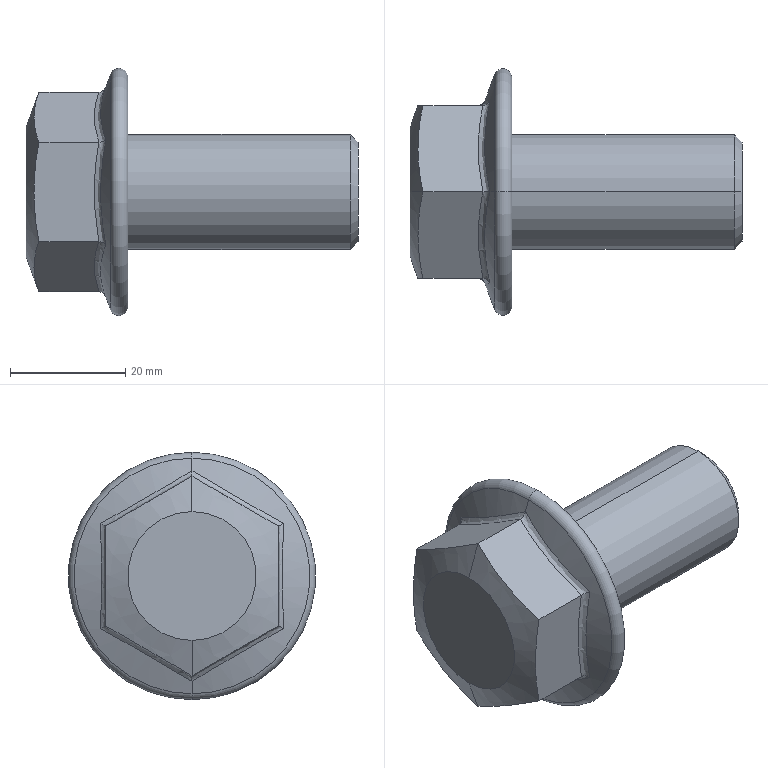Part | SolidWorks | features Fillet 2, RevCut 2, Boss 1, Chamfer 1, Extrusion 1, LPattern 1, Revolution 1 | 1 solid | 25 faces | box 57.7 x 43 x 43 mm | volume 28324 mm3 | plane 9 | cone 6 | spline 6 | torus 2 | cylinder 2 | commonest cylinder face diameters 20 x2
STEP:
#1=CARTESIAN_POINT('',(57.7,0.,-8.647));
#2=VERTEX_POINT('',#1);
#3=CARTESIAN_POINT('',(57.7,0.,8.647));
#4=VERTEX_POINT('',#3);
#5=CARTESIAN_POINT('',(57.7,0.,0.));
#6=DIRECTION('',(1.,0.,0.));
#7=DIRECTION('',(0.,0.,-1.));
#8=AXIS2_PLACEMENT_3D('',#5,#6,#7);
#9=CIRCLE('',#8,8.647);
#10=EDGE_CURVE('',#2,#4,#9,.T.);
#11=ORIENTED_EDGE('',*,*,#10,.F.);
#12=CARTESIAN_POINT('',(56.347,0.,-10.));
#13=VERTEX_POINT('',#12);
#14=CARTESIAN_POINT('',(57.7,0.,-8.647));
#15=DIRECTION('',(-0.7071,0.,-0.7071));
#16=VECTOR('',#15,1000.);
#17=LINE('',#14,#16);
#18=EDGE_CURVE('',#2,#13,#17,.T.);
#19=ORIENTED_EDGE('',*,*,#18,.T.);
#20=CARTESIAN_POINT('',(56.347,0.,10.));
#21=VERTEX_POINT('',#20);
#22=CARTESIAN_POINT('',(56.347,0.,0.));
#23=DIRECTION('',(-1.,0.,0.));
#24=DIRECTION('',(0.,0.,-1.));
#25=AXIS2_PLACEMENT_3D('',#22,#23,#24);
#26=CIRCLE('',#25,10.);
#27=EDGE_CURVE('',#21,#13,#26,.T.);
#28=ORIENTED_EDGE('',*,*,#27,.F.);
#29=CARTESIAN_POINT('',(57.7,0.,8.647));
#30=DIRECTION('',(-0.7071,0.,0.7071));
#31=VECTOR('',#30,1000.);
#32=LINE('',#29,#31);
#33=EDGE_CURVE('',#4,#21,#32,.T.);
#34=ORIENTED_EDGE('',*,*,#33,.F.);
#35=EDGE_LOOP('',(#11,#19,#28,#34));
#36=FACE_OUTER_BOUND('',#35,.T.);
#37=CARTESIAN_POINT('',(57.7,0.,0.));
#38=DIRECTION('',(-1.,0.,0.));
#39=DIRECTION('',(0.,0.,1.));
#40=AXIS2_PLACEMENT_3D('',#37,#38,#39);
#41=CONICAL_SURFACE('',#40,8.647,0.7854);
#42=ADVANCED_FACE('',(#36),#41,.T.);
#43=CARTESIAN_POINT('',(0.,0.,11.2));
#44=VERTEX_POINT('',#43);
#45=CARTESIAN_POINT('',(0.,0.,-11.2));
#46=VERTEX_POINT('',#45);
#47=CARTESIAN_POINT('',(0.,0.,0.));
#48=DIRECTION('',(-1.,0.,0.));
#49=DIRECTION('',(0.,0.,1.));
#50=AXIS2_PLACEMENT_3D('',#47,#48,#49);
#51=CIRCLE('',#50,11.2);
#52=EDGE_CURVE('',#44,#46,#51,.T.);
#53=ORIENTED_EDGE('',*,*,#52,.F.);
#54=CARTESIAN_POINT('',(2.228,0.,17.321));
#55=VERTEX_POINT('',#54);
#56=CARTESIAN_POINT('',(0.,0.,11.2));
#57=DIRECTION('',(0.342,0.,0.9397));
#58=VECTOR('',#57,1000.);
#59=LINE('',#56,#58);
#60=EDGE_CURVE('',#44,#55,#59,.T.);
#61=ORIENTED_EDGE('',*,*,#60,.T.);
#62=CARTESIAN_POINT('',(2.228,15.,8.66));
#63=VERTEX_POINT('',#62);
#64=CARTESIAN_POINT('',(2.228,0.,17.321));
#65=CARTESIAN_POINT('',(1.965,1.25,16.599));
#66=CARTESIAN_POINT('',(1.752,2.5,15.877));
#67=CARTESIAN_POINT('',(1.46,5.,14.434));
#68=CARTESIAN_POINT('',(1.306,7.5,12.99));
#69=CARTESIAN_POINT('',(1.46,10.,11.547));
#70=CARTESIAN_POINT('',(1.752,12.5,10.104));
#71=CARTESIAN_POINT('',(1.965,13.75,9.382));
#72=CARTESIAN_POINT('',(2.228,15.,8.66));
#73=B_SPLINE_CURVE_WITH_KNOTS('',3,(#64,#65,#66,#67,#68,#69,#70,#71,#72),.UNSPECIFIED.,.F.,.F.,(4,2,1,2,4),(0.000000231,0.00433,0.00866,0.01299,0.01732),.UNSPECIFIED.);
#74=EDGE_CURVE('',#55,#63,#73,.T.);
#75=ORIENTED_EDGE('',*,*,#74,.T.);
#76=CARTESIAN_POINT('',(2.228,15.,-8.66));
#77=VERTEX_POINT('',#76);
#78=CARTESIAN_POINT('',(2.228,15.,8.66));
#79=CARTESIAN_POINT('',(1.966,15.,7.223));
#80=CARTESIAN_POINT('',(1.753,15.,5.782));
#81=CARTESIAN_POINT('',(1.461,15.,2.9));
#82=CARTESIAN_POINT('',(1.384,15.,1.458));
#83=CARTESIAN_POINT('',(1.383,15.,-1.431));
#84=CARTESIAN_POINT('',(1.46,15.,-2.877));
#85=CARTESIAN_POINT('',(1.751,15.,-5.773));
#86=CARTESIAN_POINT('',(1.966,15.,-7.224));
#87=CARTESIAN_POINT('',(2.228,15.,-8.66));
#88=B_SPLINE_CURVE_WITH_KNOTS('',3,(#78,#79,#80,#81,#82,#83,#84,#85,#86,#87),.UNSPECIFIED.,.F.,.F.,(4,2,2,2,4),(0.0319,0.03626,0.04061,0.04497,0.04933),.UNSPECIFIED.);
#89=EDGE_CURVE('',#63,#77,#88,.T.);
#90=ORIENTED_EDGE('',*,*,#89,.T.);
#91=CARTESIAN_POINT('',(2.228,0.,-17.321));
#92=VERTEX_POINT('',#91);
#93=CARTESIAN_POINT('',(2.228,15.,-8.66));
#94=CARTESIAN_POINT('',(1.965,13.75,-9.382));
#95=CARTESIAN_POINT('',(1.752,12.5,-10.104));
#96=CARTESIAN_POINT('',(1.46,10.,-11.547));
#97=CARTESIAN_POINT('',(1.306,7.5,-12.99));
#98=CARTESIAN_POINT('',(1.46,5.,-14.434));
#99=CARTESIAN_POINT('',(1.752,2.5,-15.877));
#100=CARTESIAN_POINT('',(1.965,1.25,-16.599));
#101=CARTESIAN_POINT('',(2.228,0.,-17.321));
#102=B_SPLINE_CURVE_WITH_KNOTS('',3,(#93,#94,#95,#96,#97,#98,#99,#100,#101),.UNSPECIFIED.,.F.,.F.,(4,2,1,2,4),(0.000000231,0.00433,0.00866,0.01299,0.01732),.UNSPECIFIED.);
#103=EDGE_CURVE('',#77,#92,#102,.T.);
#104=ORIENTED_EDGE('',*,*,#103,.T.);
#105=CARTESIAN_POINT('',(0.,0.,-11.2));
#106=DIRECTION('',(0.342,0.,-0.9397));
#107=VECTOR('',#106,1000.);
#108=LINE('',#105,#107);
#109=EDGE_CURVE('',#46,#92,#108,.T.);
#110=ORIENTED_EDGE('',*,*,#109,.F.);
#111=EDGE_LOOP('',(#53,#61,#75,#90,#104,#110));
#112=FACE_OUTER_BOUND('',#111,.T.);
#113=CARTESIAN_POINT('',(0.,0.,0.));
#114=DIRECTION('',(1.,0.,0.));
#115=DIRECTION('',(0.,0.,-1.));
#116=AXIS2_PLACEMENT_3D('',#113,#114,#115);
#117=CONICAL_SURFACE('',#116,11.2,1.222);
#118=ADVANCED_FACE('',(#112),#117,.T.);
#119=CARTESIAN_POINT('',(14.7,0.,-20.482));
#120=VERTEX_POINT('',#119);
#121=CARTESIAN_POINT('',(14.7,0.,20.482));
#122=VERTEX_POINT('',#121);
#123=CARTESIAN_POINT('',(14.7,0.,0.));
#124=DIRECTION('',(1.,0.,0.));
#125=DIRECTION('',(0.,0.,-1.));
#126=AXIS2_PLACEMENT_3D('',#123,#124,#125);
#127=CIRCLE('',#126,20.482);
#128=EDGE_CURVE('',#120,#122,#127,.T.);
#129=ORIENTED_EDGE('',*,*,#128,.T.);
#130=CARTESIAN_POINT('',(17.7,0.,19.953));
#131=VERTEX_POINT('',#130);
#132=CARTESIAN_POINT('',(16.153,0.,19.953));
#133=DIRECTION('',(0.,1.,0.));
#134=DIRECTION('',(0.,0.,1.));
#135=AXIS2_PLACEMENT_3D('',#132,#133,#134);
#136=CIRCLE('',#135,1.547);
#137=EDGE_CURVE('',#122,#131,#136,.T.);
#138=ORIENTED_EDGE('',*,*,#137,.T.);
#139=CARTESIAN_POINT('',(17.7,0.,-19.953));
#140=VERTEX_POINT('',#139);
#141=CARTESIAN_POINT('',(17.7,0.,0.));
#142=DIRECTION('',(1.,0.,0.));
#143=DIRECTION('',(0.,0.,-1.));
#144=AXIS2_PLACEMENT_3D('',#141,#142,#143);
#145=CIRCLE('',#144,19.953);
#146=EDGE_CURVE('',#140,#131,#145,.T.);
#147=ORIENTED_EDGE('',*,*,#146,.F.);
#148=CARTESIAN_POINT('',(16.153,0.,-19.953));
#149=DIRECTION('',(0.,-1.,0.));
#150=DIRECTION('',(0.,0.,-1.));
#151=AXIS2_PLACEMENT_3D('',#148,#149,#150);
#152=CIRCLE('',#151,1.547);
#153=EDGE_CURVE('',#120,#140,#152,.T.);
#154=ORIENTED_EDGE('',*,*,#153,.F.);
#155=EDGE_LOOP('',(#129,#138,#147,#154));
#156=FACE_OUTER_BOUND('',#155,.T.);
#157=CARTESIAN_POINT('',(16.153,0.,0.));
#158=DIRECTION('',(1.,0.,0.));
#159=DIRECTION('',(0.,0.,-1.));
#160=AXIS2_PLACEMENT_3D('',#157,#158,#159);
#161=TOROIDAL_SURFACE('',#160,19.953,1.547);
#162=ADVANCED_FACE('',(#156),#161,.T.);
#163=CARTESIAN_POINT('',(13.904,15.845,9.148));
#164=VERTEX_POINT('',#163);
#165=CARTESIAN_POINT('',(13.904,0.,18.296));
#166=VERTEX_POINT('',#165);
#167=CARTESIAN_POINT('',(13.904,15.845,9.148));
#168=CARTESIAN_POINT('',(13.625,14.53,9.89));
#169=CARTESIAN_POINT('',(13.395,13.211,10.636));
#170=CARTESIAN_POINT('',(13.078,10.565,12.14));
#171=CARTESIAN_POINT('',(12.992,9.237,12.899));
#172=CARTESIAN_POINT('',(12.992,6.574,14.437));
#173=CARTESIAN_POINT('',(13.077,5.248,15.209));
#174=CARTESIAN_POINT('',(13.394,2.61,16.756));
#175=CARTESIAN_POINT('',(13.624,1.302,17.527));
#176=CARTESIAN_POINT('',(13.904,0.,18.296));
#177=B_SPLINE_CURVE_WITH_KNOTS('',3,(#167,#168,#169,#170,#171,#172,#173,#174,#175,#176),.UNSPECIFIED.,.F.,.F.,(4,2,2,2,4),(0.,0.004591,0.009181,0.01377,0.01836),.UNSPECIFIED.);
#178=EDGE_CURVE('',#164,#166,#177,.T.);
#179=ORIENTED_EDGE('',*,*,#178,.T.);
#180=CARTESIAN_POINT('',(14.7,0.,20.482));
#181=DIRECTION('',(0.342,0.,0.9397));
#182=VECTOR('',#181,1000.);
#183=LINE('',#180,#182);
#184=EDGE_CURVE('',#166,#122,#183,.T.);
#185=ORIENTED_EDGE('',*,*,#184,.T.);
#186=ORIENTED_EDGE('',*,*,#128,.F.);
#187=CARTESIAN_POINT('',(13.904,0.,-18.296));
#188=VERTEX_POINT('',#187);
#189=CARTESIAN_POINT('',(14.7,0.,-20.482));
#190=DIRECTION('',(0.342,0.,-0.9397));
#191=VECTOR('',#190,1000.);
#192=LINE('',#189,#191);
#193=EDGE_CURVE('',#188,#120,#192,.T.);
#194=ORIENTED_EDGE('',*,*,#193,.F.);
#195=CARTESIAN_POINT('',(13.904,15.845,-9.148));
#196=VERTEX_POINT('',#195);
#197=CARTESIAN_POINT('',(13.904,0.,-18.296));
#198=CARTESIAN_POINT('',(13.625,1.3,-17.528));
#199=CARTESIAN_POINT('',(13.395,2.605,-16.759));
#200=CARTESIAN_POINT('',(13.078,5.231,-15.219));
#201=CARTESIAN_POINT('',(12.992,6.552,-14.449));
#202=CARTESIAN_POINT('',(12.992,9.216,-12.911));
#203=CARTESIAN_POINT('',(13.077,10.547,-12.15));
#204=CARTESIAN_POINT('',(13.394,13.206,-10.638));
#205=CARTESIAN_POINT('',(13.624,14.528,-9.891));
#206=CARTESIAN_POINT('',(13.904,15.845,-9.148));
#207=B_SPLINE_CURVE_WITH_KNOTS('',3,(#197,#198,#199,#200,#201,#202,#203,#204,#205,#206),.UNSPECIFIED.,.F.,.F.,(4,2,2,2,4),(0.,0.004591,0.009181,0.01377,0.01836),.UNSPECIFIED.);
#208=EDGE_CURVE('',#188,#196,#207,.T.);
#209=ORIENTED_EDGE('',*,*,#208,.T.);
#210=CARTESIAN_POINT('',(13.904,15.845,-9.148));
#211=CARTESIAN_POINT('',(13.625,15.83,-7.638));
#212=CARTESIAN_POINT('',(13.395,15.816,-6.123));
#213=CARTESIAN_POINT('',(13.078,15.796,-3.079));
#214=CARTESIAN_POINT('',(12.992,15.79,-1.55));
#215=CARTESIAN_POINT('',(12.992,15.79,1.525));
#216=CARTESIAN_POINT('',(13.077,15.796,3.059));
#217=CARTESIAN_POINT('',(13.394,15.816,6.118));
#218=CARTESIAN_POINT('',(13.624,15.83,7.636));
#219=CARTESIAN_POINT('',(13.904,15.845,9.148));
#220=B_SPLINE_CURVE_WITH_KNOTS('',3,(#210,#211,#212,#213,#214,#215,#216,#217,#218,#219),.UNSPECIFIED.,.F.,.F.,(4,2,2,2,4),(0.,0.00459,0.009181,0.01377,0.01836),.UNSPECIFIED.);
#221=EDGE_CURVE('',#196,#164,#220,.T.);
#222=ORIENTED_EDGE('',*,*,#221,.T.);
#223=EDGE_LOOP('',(#179,#185,#186,#194,#209,#222));
#224=FACE_OUTER_BOUND('',#223,.T.);
#225=CARTESIAN_POINT('',(14.7,0.,0.));
#226=DIRECTION('',(1.,0.,0.));
#227=DIRECTION('',(0.,0.,-1.));
#228=AXIS2_PLACEMENT_3D('',#225,#226,#227);
#229=CONICAL_SURFACE('',#228,20.482,1.222);
#230=ADVANCED_FACE('',(#224),#229,.T.);
#231=ORIENTED_EDGE('',*,*,#27,.T.);
#232=CARTESIAN_POINT('',(17.7,0.,-10.));
#233=VERTEX_POINT('',#232);
#234=CARTESIAN_POINT('',(57.7,0.,-10.));
#235=DIRECTION('',(-1.,0.,0.));
#236=VECTOR('',#235,1000.);
#237=LINE('',#234,#236);
#238=EDGE_CURVE('',#13,#233,#237,.T.);
#239=ORIENTED_EDGE('',*,*,#238,.T.);
#240=CARTESIAN_POINT('',(17.7,0.,10.));
#241=VERTEX_POINT('',#240);
#242=CARTESIAN_POINT('',(17.7,0.,0.));
#243=DIRECTION('',(1.,0.,0.));
#244=DIRECTION('',(0.,0.,-1.));
#245=AXIS2_PLACEMENT_3D('',#242,#243,#244);
#246=CIRCLE('',#245,10.);
#247=EDGE_CURVE('',#233,#241,#246,.T.);
#248=ORIENTED_EDGE('',*,*,#247,.T.);
#249=CARTESIAN_POINT('',(57.7,0.,10.));
#250=DIRECTION('',(-1.,0.,0.));
#251=VECTOR('',#250,1000.);
#252=LINE('',#249,#251);
#253=EDGE_CURVE('',#21,#241,#252,.T.);
#254=ORIENTED_EDGE('',*,*,#253,.F.);
#255=EDGE_LOOP('',(#231,#239,#248,#254));
#256=FACE_OUTER_BOUND('',#255,.T.);
#257=CARTESIAN_POINT('',(57.7,0.,0.));
#258=DIRECTION('',(-1.,0.,0.));
#259=DIRECTION('',(0.,0.,1.));
#260=AXIS2_PLACEMENT_3D('',#257,#258,#259);
#261=CYLINDRICAL_SURFACE('',#260,10.);
#262=ADVANCED_FACE('',(#256),#261,.T.);
#263=CARTESIAN_POINT('',(17.7,0.,0.));
#264=DIRECTION('',(1.,0.,0.));
#265=DIRECTION('',(0.,0.,-1.));
#266=AXIS2_PLACEMENT_3D('',#263,#264,#265);
#267=CIRCLE('',#266,10.);
#268=EDGE_CURVE('',#241,#233,#267,.T.);
#269=ORIENTED_EDGE('',*,*,#268,.F.);
#270=ORIENTED_EDGE('',*,*,#247,.F.);
#271=EDGE_LOOP('',(#269,#270));
#272=FACE_BOUND('',#271,.T.);
#273=ORIENTED_EDGE('',*,*,#146,.T.);
#274=CARTESIAN_POINT('',(17.7,0.,0.));
#275=DIRECTION('',(1.,0.,0.));
#276=DIRECTION('',(0.,0.,-1.));
#277=AXIS2_PLACEMENT_3D('',#274,#275,#276);
#278=CIRCLE('',#277,19.953);
#279=EDGE_CURVE('',#131,#140,#278,.T.);
#280=ORIENTED_EDGE('',*,*,#279,.T.);
#281=EDGE_LOOP('',(#273,#280));
#282=FACE_OUTER_BOUND('',#281,.T.);
#283=CARTESIAN_POINT('',(17.7,0.,-17.321));
#284=DIRECTION('',(1.,0.,0.));
#285=DIRECTION('',(0.,0.,-1.));
#286=AXIS2_PLACEMENT_3D('',#283,#284,#285);
#287=PLANE('',#286);
#288=ADVANCED_FACE('',(#272,#282),#287,.T.);
#289=ORIENTED_EDGE('',*,*,#238,.F.);
#290=CARTESIAN_POINT('',(56.347,0.,0.));
#291=DIRECTION('',(-1.,0.,0.));
#292=DIRECTION('',(0.,0.,-1.));
#293=AXIS2_PLACEMENT_3D('',#290,#291,#292);
#294=CIRCLE('',#293,10.);
#295=EDGE_CURVE('',#13,#21,#294,.T.);
#296=ORIENTED_EDGE('',*,*,#295,.T.);
#297=ORIENTED_EDGE('',*,*,#253,.T.);
#298=ORIENTED_EDGE('',*,*,#268,.T.);
#299=EDGE_LOOP('',(#289,#296,#297,#298));
#300=FACE_OUTER_BOUND('',#299,.T.);
#301=CARTESIAN_POINT('',(57.7,0.,0.));
#302=DIRECTION('',(-1.,0.,0.));
#303=DIRECTION('',(0.,0.,1.));
#304=AXIS2_PLACEMENT_3D('',#301,#302,#303);
#305=CYLINDRICAL_SURFACE('',#304,10.);
#306=ADVANCED_FACE('',(#300),#305,.T.);
#307=CARTESIAN_POINT('',(57.7,0.,0.));
#308=DIRECTION('',(1.,0.,0.));
#309=DIRECTION('',(0.,0.,-1.));
#310=AXIS2_PLACEMENT_3D('',#307,#308,#309);
#311=CIRCLE('',#310,8.647);
#312=EDGE_CURVE('',#4,#2,#311,.T.);
#313=ORIENTED_EDGE('',*,*,#312,.T.);
#314=ORIENTED_EDGE('',*,*,#10,.T.);
#315=EDGE_LOOP('',(#313,#314));
#316=FACE_OUTER_BOUND('',#315,.T.);
#317=CARTESIAN_POINT('',(57.7,0.,0.));
#318=DIRECTION('',(1.,0.,0.));
#319=DIRECTION('',(0.,0.,-1.));
#320=AXIS2_PLACEMENT_3D('',#317,#318,#319);
#321=PLANE('',#320);
#322=ADVANCED_FACE('',(#316),#321,.T.);
#323=ORIENTED_EDGE('',*,*,#184,.F.);
#324=CARTESIAN_POINT('',(13.904,-15.845,9.148));
#325=VERTEX_POINT('',#324);
#326=CARTESIAN_POINT('',(13.904,0.,18.296));
#327=CARTESIAN_POINT('',(13.625,-1.3,17.528));
#328=CARTESIAN_POINT('',(13.395,-2.605,16.759));
#329=CARTESIAN_POINT('',(13.078,-5.231,15.219));
#330=CARTESIAN_POINT('',(12.992,-6.552,14.449));
#331=CARTESIAN_POINT('',(12.992,-9.216,12.911));
#332=CARTESIAN_POINT('',(13.077,-10.547,12.15));
#333=CARTESIAN_POINT('',(13.394,-13.206,10.638));
#334=CARTESIAN_POINT('',(13.624,-14.528,9.891));
#335=CARTESIAN_POINT('',(13.904,-15.845,9.148));
#336=B_SPLINE_CURVE_WITH_KNOTS('',3,(#326,#327,#328,#329,#330,#331,#332,#333,#334,#335),.UNSPECIFIED.,.F.,.F.,(4,2,2,2,4),(0.,0.004591,0.009181,0.01377,0.01836),.UNSPECIFIED.);
#337=EDGE_CURVE('',#166,#325,#336,.T.);
#338=ORIENTED_EDGE('',*,*,#337,.T.);
#339=CARTESIAN_POINT('',(13.904,-15.845,-9.148));
#340=VERTEX_POINT('',#339);
#341=CARTESIAN_POINT('',(13.904,-15.845,9.148));
#342=CARTESIAN_POINT('',(13.625,-15.83,7.638));
#343=CARTESIAN_POINT('',(13.395,-15.816,6.123));
#344=CARTESIAN_POINT('',(13.078,-15.796,3.079));
#345=CARTESIAN_POINT('',(12.992,-15.79,1.55));
#346=CARTESIAN_POINT('',(12.992,-15.79,-1.525));
#347=CARTESIAN_POINT('',(13.077,-15.796,-3.06));
#348=CARTESIAN_POINT('',(13.394,-15.816,-6.118));
#349=CARTESIAN_POINT('',(13.624,-15.83,-7.636));
#350=CARTESIAN_POINT('',(13.904,-15.845,-9.148));
#351=B_SPLINE_CURVE_WITH_KNOTS('',3,(#341,#342,#343,#344,#345,#346,#347,#348,#349,#350),.UNSPECIFIED.,.F.,.F.,(4,2,2,2,4),(0.,0.004591,0.009181,0.01377,0.01836),.UNSPECIFIED.);
#352=EDGE_CURVE('',#325,#340,#351,.T.);
#353=ORIENTED_EDGE('',*,*,#352,.T.);
#354=CARTESIAN_POINT('',(13.904,-15.845,-9.148));
#355=CARTESIAN_POINT('',(13.625,-14.53,-9.89));
#356=CARTESIAN_POINT('',(13.395,-13.211,-10.636));
#357=CARTESIAN_POINT('',(13.078,-10.565,-12.14));
#358=CARTESIAN_POINT('',(12.992,-9.237,-12.899));
#359=CARTESIAN_POINT('',(12.992,-6.574,-14.437));
#360=CARTESIAN_POINT('',(13.077,-5.248,-15.209));
#361=CARTESIAN_POINT('',(13.394,-2.61,-16.756));
#362=CARTESIAN_POINT('',(13.624,-1.302,-17.527));
#363=CARTESIAN_POINT('',(13.904,0.,-18.296));
#364=B_SPLINE_CURVE_WITH_KNOTS('',3,(#354,#355,#356,#357,#358,#359,#360,#361,#362,#363),.UNSPECIFIED.,.F.,.F.,(4,2,2,2,4),(0.,0.004591,0.009181,0.01377,0.01836),.UNSPECIFIED.);
#365=EDGE_CURVE('',#340,#188,#364,.T.);
#366=ORIENTED_EDGE('',*,*,#365,.T.);
#367=ORIENTED_EDGE('',*,*,#193,.T.);
#368=CARTESIAN_POINT('',(14.7,0.,0.));
#369=DIRECTION('',(1.,0.,0.));
#370=DIRECTION('',(0.,0.,-1.));
#371=AXIS2_PLACEMENT_3D('',#368,#369,#370);
#372=CIRCLE('',#371,20.482);
#373=EDGE_CURVE('',#122,#120,#372,.T.);
#374=ORIENTED_EDGE('',*,*,#373,.F.);
#375=EDGE_LOOP('',(#323,#338,#353,#366,#367,#374));
#376=FACE_OUTER_BOUND('',#375,.T.);
#377=CARTESIAN_POINT('',(14.7,0.,0.));
#378=DIRECTION('',(1.,0.,0.));
#379=DIRECTION('',(0.,0.,-1.));
#380=AXIS2_PLACEMENT_3D('',#377,#378,#379);
#381=CONICAL_SURFACE('',#380,20.482,1.222);
#382=ADVANCED_FACE('',(#376),#381,.T.);
#383=ORIENTED_EDGE('',*,*,#137,.F.);
#384=ORIENTED_EDGE('',*,*,#373,.T.);
#385=ORIENTED_EDGE('',*,*,#153,.T.);
#386=ORIENTED_EDGE('',*,*,#279,.F.);
#387=EDGE_LOOP('',(#383,#384,#385,#386));
#388=FACE_OUTER_BOUND('',#387,.T.);
#389=CARTESIAN_POINT('',(16.153,0.,0.));
#390=DIRECTION('',(1.,0.,0.));
#391=DIRECTION('',(0.,0.,-1.));
#392=AXIS2_PLACEMENT_3D('',#389,#390,#391);
#393=TOROIDAL_SURFACE('',#392,19.953,1.547);
#394=ADVANCED_FACE('',(#388),#393,.T.);
#395=CARTESIAN_POINT('',(0.,0.,0.));
#396=DIRECTION('',(-1.,0.,0.));
#397=DIRECTION('',(0.,0.,1.));
#398=AXIS2_PLACEMENT_3D('',#395,#396,#397);
#399=CIRCLE('',#398,11.2);
#400=EDGE_CURVE('',#46,#44,#399,.T.);
#401=ORIENTED_EDGE('',*,*,#400,.T.);
#402=ORIENTED_EDGE('',*,*,#52,.T.);
#403=EDGE_LOOP('',(#401,#402));
#404=FACE_OUTER_BOUND('',#403,.T.);
#405=CARTESIAN_POINT('',(0.,0.,-17.321));
#406=DIRECTION('',(1.,0.,0.));
#407=DIRECTION('',(0.,0.,-1.));
#408=AXIS2_PLACEMENT_3D('',#405,#406,#407);
#409=PLANE('',#408);
#410=ADVANCED_FACE('',(#404),#409,.F.);
#411=ORIENTED_EDGE('',*,*,#60,.F.);
#412=ORIENTED_EDGE('',*,*,#400,.F.);
#413=ORIENTED_EDGE('',*,*,#109,.T.);
#414=CARTESIAN_POINT('',(2.228,-15.,-8.66));
#415=VERTEX_POINT('',#414);
#416=CARTESIAN_POINT('',(2.228,0.,-17.321));
#417=CARTESIAN_POINT('',(1.965,-1.25,-16.599));
#418=CARTESIAN_POINT('',(1.752,-2.5,-15.877));
#419=CARTESIAN_POINT('',(1.46,-5.,-14.434));
#420=CARTESIAN_POINT('',(1.306,-7.5,-12.99));
#421=CARTESIAN_POINT('',(1.46,-10.,-11.547));
#422=CARTESIAN_POINT('',(1.752,-12.5,-10.104));
#423=CARTESIAN_POINT('',(1.965,-13.75,-9.382));
#424=CARTESIAN_POINT('',(2.228,-15.,-8.66));
#425=B_SPLINE_CURVE_WITH_KNOTS('',3,(#416,#417,#418,#419,#420,#421,#422,#423,#424),.UNSPECIFIED.,.F.,.F.,(4,2,1,2,4),(0.000000231,0.00433,0.00866,0.01299,0.01732),.UNSPECIFIED.);
#426=EDGE_CURVE('',#92,#415,#425,.T.);
#427=ORIENTED_EDGE('',*,*,#426,.T.);
#428=CARTESIAN_POINT('',(2.228,-15.,8.66));
#429=VERTEX_POINT('',#428);
#430=CARTESIAN_POINT('',(2.228,-15.,-8.66));
#431=CARTESIAN_POINT('',(1.966,-15.,-7.224));
#432=CARTESIAN_POINT('',(1.751,-15.,-5.773));
#433=CARTESIAN_POINT('',(1.46,-15.,-2.877));
#434=CARTESIAN_POINT('',(1.383,-15.,-1.431));
#435=CARTESIAN_POINT('',(1.384,-15.,1.458));
#436=CARTESIAN_POINT('',(1.461,-15.,2.9));
#437=CARTESIAN_POINT('',(1.753,-15.,5.782));
#438=CARTESIAN_POINT('',(1.966,-15.,7.223));
#439=CARTESIAN_POINT('',(2.228,-15.,8.66));
#440=B_SPLINE_CURVE_WITH_KNOTS('',3,(#430,#431,#432,#433,#434,#435,#436,#437,#438,#439),.UNSPECIFIED.,.F.,.F.,(4,2,2,2,4),(0.01459,0.01897,0.02334,0.02771,0.03208),.UNSPECIFIED.);
#441=EDGE_CURVE('',#415,#429,#440,.T.);
#442=ORIENTED_EDGE('',*,*,#441,.T.);
#443=CARTESIAN_POINT('',(2.228,-15.,8.66));
#444=CARTESIAN_POINT('',(1.965,-13.75,9.382));
#445=CARTESIAN_POINT('',(1.752,-12.5,10.104));
#446=CARTESIAN_POINT('',(1.46,-10.,11.547));
#447=CARTESIAN_POINT('',(1.306,-7.5,12.99));
#448=CARTESIAN_POINT('',(1.46,-5.,14.434));
#449=CARTESIAN_POINT('',(1.752,-2.5,15.877));
#450=CARTESIAN_POINT('',(1.965,-1.25,16.599));
#451=CARTESIAN_POINT('',(2.228,0.,17.321));
#452=B_SPLINE_CURVE_WITH_KNOTS('',3,(#443,#444,#445,#446,#447,#448,#449,#450,#451),.UNSPECIFIED.,.F.,.F.,(4,2,1,2,4),(0.000000231,0.00433,0.00866,0.01299,0.01732),.UNSPECIFIED.);
#453=EDGE_CURVE('',#429,#55,#452,.T.);
#454=ORIENTED_EDGE('',*,*,#453,.T.);
#455=EDGE_LOOP('',(#411,#412,#413,#427,#442,#454));
#456=FACE_OUTER_BOUND('',#455,.T.);
#457=CARTESIAN_POINT('',(0.,0.,0.));
#458=DIRECTION('',(1.,0.,0.));
#459=DIRECTION('',(0.,0.,-1.));
#460=AXIS2_PLACEMENT_3D('',#457,#458,#459);
#461=CONICAL_SURFACE('',#460,11.2,1.222);
#462=ADVANCED_FACE('',(#456),#461,.T.);
#463=CARTESIAN_POINT('',(12.654,-15.,-8.66));
#464=VERTEX_POINT('',#463);
#465=CARTESIAN_POINT('',(17.7,-15.,-8.66));
#466=DIRECTION('',(-1.,0.,0.));
#467=VECTOR('',#466,1000.);
#468=LINE('',#465,#467);
#469=EDGE_CURVE('',#464,#415,#468,.T.);
#470=ORIENTED_EDGE('',*,*,#469,.F.);
#471=CARTESIAN_POINT('',(12.654,-15.,8.66));
#472=VERTEX_POINT('',#471);
#473=CARTESIAN_POINT('',(12.654,-15.,-8.66));
#474=CARTESIAN_POINT('',(12.408,-15.,-7.227));
#475=CARTESIAN_POINT('',(12.209,-15.,-5.79));
#476=CARTESIAN_POINT('',(11.937,-15.,-2.904));
#477=CARTESIAN_POINT('',(11.864,-15.,-1.455));
#478=CARTESIAN_POINT('',(11.864,-15.,1.455));
#479=CARTESIAN_POINT('',(11.937,-15.,2.904));
#480=CARTESIAN_POINT('',(12.209,-15.,5.79));
#481=CARTESIAN_POINT('',(12.408,-15.,7.227));
#482=CARTESIAN_POINT('',(12.654,-15.,8.66));
#483=B_SPLINE_CURVE_WITH_KNOTS('',3,(#473,#474,#475,#476,#477,#478,#479,#480,#481,#482),.UNSPECIFIED.,.F.,.F.,(4,2,2,2,4),(0.,0.004348,0.008696,0.01304,0.01739),.UNSPECIFIED.);
#484=EDGE_CURVE('',#464,#472,#483,.T.);
#485=ORIENTED_EDGE('',*,*,#484,.T.);
#486=CARTESIAN_POINT('',(17.7,-15.,8.66));
#487=DIRECTION('',(-1.,0.,0.));
#488=VECTOR('',#487,1000.);
#489=LINE('',#486,#488);
#490=EDGE_CURVE('',#472,#429,#489,.T.);
#491=ORIENTED_EDGE('',*,*,#490,.T.);
#492=ORIENTED_EDGE('',*,*,#441,.F.);
#493=EDGE_LOOP('',(#470,#485,#491,#492));
#494=FACE_OUTER_BOUND('',#493,.T.);
#495=CARTESIAN_POINT('',(17.7,-15.,8.66));
#496=DIRECTION('',(0.,1.,0.));
#497=DIRECTION('',(0.,0.,1.));
#498=AXIS2_PLACEMENT_3D('',#495,#496,#497);
#499=PLANE('',#498);
#500=ADVANCED_FACE('',(#494),#499,.F.);
#501=ORIENTED_EDGE('',*,*,#490,.F.);
#502=CARTESIAN_POINT('',(12.654,0.,17.321));
#503=VERTEX_POINT('',#502);
#504=CARTESIAN_POINT('',(12.654,-15.,8.66));
#505=CARTESIAN_POINT('',(12.408,-13.759,9.377));
#506=CARTESIAN_POINT('',(12.209,-12.514,10.095));
#507=CARTESIAN_POINT('',(11.937,-10.015,11.538));
#508=CARTESIAN_POINT('',(11.864,-8.76,12.263));
#509=CARTESIAN_POINT('',(11.864,-6.24,13.718));
#510=CARTESIAN_POINT('',(11.937,-4.985,14.442));
#511=CARTESIAN_POINT('',(12.209,-2.486,15.885));
#512=CARTESIAN_POINT('',(12.408,-1.241,16.604));
#513=CARTESIAN_POINT('',(12.654,0.,17.321));
#514=B_SPLINE_CURVE_WITH_KNOTS('',3,(#504,#505,#506,#507,#508,#509,#510,#511,#512,#513),.UNSPECIFIED.,.F.,.F.,(4,2,2,2,4),(0.,0.004348,0.008696,0.01304,0.01739),.UNSPECIFIED.);
#515=EDGE_CURVE('',#472,#503,#514,.T.);
#516=ORIENTED_EDGE('',*,*,#515,.T.);
#517=CARTESIAN_POINT('',(17.7,0.,17.321));
#518=DIRECTION('',(-1.,0.,0.));
#519=VECTOR('',#518,1000.);
#520=LINE('',#517,#519);
#521=EDGE_CURVE('',#503,#55,#520,.T.);
#522=ORIENTED_EDGE('',*,*,#521,.T.);
#523=ORIENTED_EDGE('',*,*,#453,.F.);
#524=EDGE_LOOP('',(#501,#516,#522,#523));
#525=FACE_OUTER_BOUND('',#524,.T.);
#526=CARTESIAN_POINT('',(17.7,0.,17.321));
#527=DIRECTION('',(0.,0.5,-0.866));
#528=DIRECTION('',(0.,0.866,0.5));
#529=AXIS2_PLACEMENT_3D('',#526,#527,#528);
#530=PLANE('',#529);
#531=ADVANCED_FACE('',(#525),#530,.F.);
#532=ORIENTED_EDGE('',*,*,#521,.F.);
#533=CARTESIAN_POINT('',(12.654,15.,8.66));
#534=VERTEX_POINT('',#533);
#535=CARTESIAN_POINT('',(12.654,0.,17.321));
#536=CARTESIAN_POINT('',(12.408,1.241,16.604));
#537=CARTESIAN_POINT('',(12.209,2.486,15.885));
#538=CARTESIAN_POINT('',(11.937,4.985,14.442));
#539=CARTESIAN_POINT('',(11.864,6.24,13.718));
#540=CARTESIAN_POINT('',(11.864,8.76,12.263));
#541=CARTESIAN_POINT('',(11.937,10.015,11.538));
#542=CARTESIAN_POINT('',(12.209,12.514,10.095));
#543=CARTESIAN_POINT('',(12.408,13.759,9.377));
#544=CARTESIAN_POINT('',(12.654,15.,8.66));
#545=B_SPLINE_CURVE_WITH_KNOTS('',3,(#535,#536,#537,#538,#539,#540,#541,#542,#543,#544),.UNSPECIFIED.,.F.,.F.,(4,2,2,2,4),(0.,0.004348,0.008696,0.01304,0.01739),.UNSPECIFIED.);
#546=EDGE_CURVE('',#503,#534,#545,.T.);
#547=ORIENTED_EDGE('',*,*,#546,.T.);
#548=CARTESIAN_POINT('',(17.7,15.,8.66));
#549=DIRECTION('',(-1.,0.,0.));
#550=VECTOR('',#549,1000.);
#551=LINE('',#548,#550);
#552=EDGE_CURVE('',#534,#63,#551,.T.);
#553=ORIENTED_EDGE('',*,*,#552,.T.);
#554=ORIENTED_EDGE('',*,*,#74,.F.);
#555=EDGE_LOOP('',(#532,#547,#553,#554));
#556=FACE_OUTER_BOUND('',#555,.T.);
#557=CARTESIAN_POINT('',(17.7,15.,8.66));
#558=DIRECTION('',(0.,-0.5,-0.866));
#559=DIRECTION('',(0.,0.866,-0.5));
#560=AXIS2_PLACEMENT_3D('',#557,#558,#559);
#561=PLANE('',#560);
#562=ADVANCED_FACE('',(#556),#561,.F.);
#563=ORIENTED_EDGE('',*,*,#552,.F.);
#564=CARTESIAN_POINT('',(12.654,15.,-8.66));
#565=VERTEX_POINT('',#564);
#566=CARTESIAN_POINT('',(12.654,15.,8.66));
#567=CARTESIAN_POINT('',(12.408,15.,7.227));
#568=CARTESIAN_POINT('',(12.209,15.,5.79));
#569=CARTESIAN_POINT('',(11.937,15.,2.904));
#570=CARTESIAN_POINT('',(11.864,15.,1.455));
#571=CARTESIAN_POINT('',(11.864,15.,-1.455));
#572=CARTESIAN_POINT('',(11.937,15.,-2.904));
#573=CARTESIAN_POINT('',(12.209,15.,-5.79));
#574=CARTESIAN_POINT('',(12.408,15.,-7.227));
#575=CARTESIAN_POINT('',(12.654,15.,-8.66));
#576=B_SPLINE_CURVE_WITH_KNOTS('',3,(#566,#567,#568,#569,#570,#571,#572,#573,#574,#575),.UNSPECIFIED.,.F.,.F.,(4,2,2,2,4),(0.,0.004348,0.008696,0.01304,0.01739),.UNSPECIFIED.);
#577=EDGE_CURVE('',#534,#565,#576,.T.);
#578=ORIENTED_EDGE('',*,*,#577,.T.);
#579=CARTESIAN_POINT('',(17.7,15.,-8.66));
#580=DIRECTION('',(-1.,0.,0.));
#581=VECTOR('',#580,1000.);
#582=LINE('',#579,#581);
#583=EDGE_CURVE('',#565,#77,#582,.T.);
#584=ORIENTED_EDGE('',*,*,#583,.T.);
#585=ORIENTED_EDGE('',*,*,#89,.F.);
#586=EDGE_LOOP('',(#563,#578,#584,#585));
#587=FACE_OUTER_BOUND('',#586,.T.);
#588=CARTESIAN_POINT('',(17.7,15.,-8.66));
#589=DIRECTION('',(0.,-1.,0.));
#590=DIRECTION('',(0.,0.,-1.));
#591=AXIS2_PLACEMENT_3D('',#588,#589,#590);
#592=PLANE('',#591);
#593=ADVANCED_FACE('',(#587),#592,.F.);
#594=ORIENTED_EDGE('',*,*,#583,.F.);
#595=CARTESIAN_POINT('',(12.654,0.,-17.321));
#596=VERTEX_POINT('',#595);
#597=CARTESIAN_POINT('',(12.654,15.,-8.66));
#598=CARTESIAN_POINT('',(12.408,13.759,-9.377));
#599=CARTESIAN_POINT('',(12.209,12.514,-10.095));
#600=CARTESIAN_POINT('',(11.937,10.015,-11.538));
#601=CARTESIAN_POINT('',(11.864,8.76,-12.263));
#602=CARTESIAN_POINT('',(11.864,6.24,-13.718));
#603=CARTESIAN_POINT('',(11.937,4.985,-14.442));
#604=CARTESIAN_POINT('',(12.209,2.486,-15.885));
#605=CARTESIAN_POINT('',(12.408,1.241,-16.604));
#606=CARTESIAN_POINT('',(12.654,0.,-17.321));
#607=B_SPLINE_CURVE_WITH_KNOTS('',3,(#597,#598,#599,#600,#601,#602,#603,#604,#605,#606),.UNSPECIFIED.,.F.,.F.,(4,2,2,2,4),(0.,0.004348,0.008696,0.01304,0.01739),.UNSPECIFIED.);
#608=EDGE_CURVE('',#565,#596,#607,.T.);
#609=ORIENTED_EDGE('',*,*,#608,.T.);
#610=CARTESIAN_POINT('',(17.7,0.,-17.321));
#611=DIRECTION('',(-1.,0.,0.));
#612=VECTOR('',#611,1000.);
#613=LINE('',#610,#612);
#614=EDGE_CURVE('',#596,#92,#613,.T.);
#615=ORIENTED_EDGE('',*,*,#614,.T.);
#616=ORIENTED_EDGE('',*,*,#103,.F.);
#617=EDGE_LOOP('',(#594,#609,#615,#616));
#618=FACE_OUTER_BOUND('',#617,.T.);
#619=CARTESIAN_POINT('',(17.7,0.,-17.321));
#620=DIRECTION('',(0.,-0.5,0.866));
#621=DIRECTION('',(0.,-0.866,-0.5));
#622=AXIS2_PLACEMENT_3D('',#619,#620,#621);
#623=PLANE('',#622);
#624=ADVANCED_FACE('',(#618),#623,.F.);
#625=ORIENTED_EDGE('',*,*,#614,.F.);
#626=CARTESIAN_POINT('',(12.654,0.,-17.321));
#627=CARTESIAN_POINT('',(12.408,-1.241,-16.604));
#628=CARTESIAN_POINT('',(12.209,-2.486,-15.885));
#629=CARTESIAN_POINT('',(11.937,-4.985,-14.442));
#630=CARTESIAN_POINT('',(11.864,-6.24,-13.718));
#631=CARTESIAN_POINT('',(11.864,-8.76,-12.263));
#632=CARTESIAN_POINT('',(11.937,-10.015,-11.538));
#633=CARTESIAN_POINT('',(12.209,-12.514,-10.095));
#634=CARTESIAN_POINT('',(12.408,-13.759,-9.377));
#635=CARTESIAN_POINT('',(12.654,-15.,-8.66));
#636=B_SPLINE_CURVE_WITH_KNOTS('',3,(#626,#627,#628,#629,#630,#631,#632,#633,#634,#635),.UNSPECIFIED.,.F.,.F.,(4,2,2,2,4),(0.,0.004348,0.008696,0.01304,0.01739),.UNSPECIFIED.);
#637=EDGE_CURVE('',#596,#464,#636,.T.);
#638=ORIENTED_EDGE('',*,*,#637,.T.);
#639=ORIENTED_EDGE('',*,*,#469,.T.);
#640=ORIENTED_EDGE('',*,*,#426,.F.);
#641=EDGE_LOOP('',(#625,#638,#639,#640));
#642=FACE_OUTER_BOUND('',#641,.T.);
#643=CARTESIAN_POINT('',(17.7,-15.,-8.66));
#644=DIRECTION('',(0.,0.5,0.866));
#645=DIRECTION('',(0.,-0.866,0.5));
#646=AXIS2_PLACEMENT_3D('',#643,#644,#645);
#647=PLANE('',#646);
#648=ADVANCED_FACE('',(#642),#647,.F.);
#649=CARTESIAN_POINT('',(13.904,0.,-18.296));
#650=CARTESIAN_POINT('',(13.808,0.,-18.032));
#651=CARTESIAN_POINT('',(13.645,0.,-17.791));
#652=CARTESIAN_POINT('',(13.209,0.,-17.434));
#653=CARTESIAN_POINT('',(12.938,0.,-17.321));
#654=CARTESIAN_POINT('',(12.654,0.,-17.321));
#655=B_SPLINE_CURVE_WITH_KNOTS('',3,(#649,#650,#651,#652,#653,#654),.UNSPECIFIED.,.F.,.F.,(4,2,4),(-0.000007277,0.0008336,0.001674),.UNSPECIFIED.);
#656=EDGE_CURVE('',#188,#596,#655,.T.);
#657=ORIENTED_EDGE('',*,*,#656,.F.);
#658=ORIENTED_EDGE('',*,*,#365,.F.);
#659=CARTESIAN_POINT('',(12.654,-15.,-8.66));
#660=CARTESIAN_POINT('',(12.938,-15.,-8.66));
#661=CARTESIAN_POINT('',(13.209,-15.098,-8.717));
#662=CARTESIAN_POINT('',(13.536,-15.33,-8.851));
#663=CARTESIAN_POINT('',(13.631,-15.421,-8.903));
#664=CARTESIAN_POINT('',(13.792,-15.622,-9.019));
#665=CARTESIAN_POINT('',(13.856,-15.731,-9.082));
#666=CARTESIAN_POINT('',(13.904,-15.845,-9.148));
#667=B_SPLINE_CURVE_WITH_KNOTS('',3,(#659,#660,#661,#662,#663,#664,#665,#666),.UNSPECIFIED.,.F.,.F.,(4,2,2,4),(0.,0.000838,0.001257,0.001676),.UNSPECIFIED.);
#668=EDGE_CURVE('',#464,#340,#667,.T.);
#669=ORIENTED_EDGE('',*,*,#668,.F.);
#670=ORIENTED_EDGE('',*,*,#637,.F.);
#671=EDGE_LOOP('',(#657,#658,#669,#670));
#672=FACE_OUTER_BOUND('',#671,.T.);
#673=CARTESIAN_POINT('',(12.796,0.6942,-17.721));
#674=CARTESIAN_POINT('',(13.667,0.5558,-17.641));
#675=CARTESIAN_POINT('',(13.924,0.09214,-18.35));
#676=CARTESIAN_POINT('',(12.516,-0.6296,-16.957));
#677=CARTESIAN_POINT('',(13.379,-0.744,-16.891));
#678=CARTESIAN_POINT('',(13.643,-1.203,-17.586));
#679=CARTESIAN_POINT('',(12.283,-1.966,-16.186));
#680=CARTESIAN_POINT('',(13.138,-2.061,-16.131));
#681=CARTESIAN_POINT('',(13.411,-2.506,-16.817));
#682=CARTESIAN_POINT('',(11.958,-4.674,-14.622));
#683=CARTESIAN_POINT('',(12.802,-4.723,-14.593));
#684=CARTESIAN_POINT('',(13.086,-5.144,-15.27));
#685=CARTESIAN_POINT('',(11.867,-6.047,-13.829));
#686=CARTESIAN_POINT('',(12.707,-6.075,-13.813));
#687=CARTESIAN_POINT('',(12.994,-6.479,-14.492));
#688=CARTESIAN_POINT('',(11.862,-8.839,-12.217));
#689=CARTESIAN_POINT('',(12.702,-8.813,-12.232));
#690=CARTESIAN_POINT('',(12.99,-9.199,-12.921));
#691=CARTESIAN_POINT('',(11.949,-10.224,-11.417));
#692=CARTESIAN_POINT('',(12.793,-10.177,-11.445));
#693=CARTESIAN_POINT('',(13.076,-10.553,-12.146));
#694=CARTESIAN_POINT('',(12.273,-12.974,-9.83));
#695=CARTESIAN_POINT('',(13.128,-12.88,-9.885));
#696=CARTESIAN_POINT('',(13.401,-13.252,-10.612));
#697=CARTESIAN_POINT('',(12.509,-14.339,-9.042));
#698=CARTESIAN_POINT('',(13.373,-14.225,-9.108));
#699=CARTESIAN_POINT('',(13.637,-14.597,-9.852));
#700=CARTESIAN_POINT('',(12.797,-15.697,-8.258));
#701=CARTESIAN_POINT('',(13.667,-15.558,-8.338));
#702=CARTESIAN_POINT('',(13.925,-15.94,-9.094));
#703=(BOUNDED_SURFACE()B_SPLINE_SURFACE(3,2,((#673,#674,#675),(#676,#677,#678),(#679,#680,#681),(#682,#683,#684),(#685,#686,#687),(#688,#689,#690),(#691,#692,#693),(#694,#695,#696),(#697,#698,#699),(#700,#701,#702)),.UNSPECIFIED.,.F.,.F.,.F.)B_SPLINE_SURFACE_WITH_KNOTS((4,2,2,2,4),(3,3),(0.07529,0.07992,0.08456,0.08919,0.09383),(0.,1.),.UNSPECIFIED.)GEOMETRIC_REPRESENTATION_ITEM()RATIONAL_B_SPLINE_SURFACE(((1.,0.8048,1.),(1.,0.8085,1.),(1.,0.8121,1.),(1.,0.8175,1.),(1.,0.8191,1.),(1.,0.8192,1.),(1.,0.8176,1.),(1.,0.8123,1.),(1.,0.8086,1.),(1.,0.8048,1.)))REPRESENTATION_ITEM('')SURFACE());
#704=ADVANCED_FACE('',(#672),#703,.F.);
#705=ORIENTED_EDGE('',*,*,#668,.T.);
#706=ORIENTED_EDGE('',*,*,#352,.F.);
#707=CARTESIAN_POINT('',(12.654,-15.,8.66));
#708=CARTESIAN_POINT('',(12.938,-15.,8.66));
#709=CARTESIAN_POINT('',(13.209,-15.098,8.717));
#710=CARTESIAN_POINT('',(13.536,-15.33,8.851));
#711=CARTESIAN_POINT('',(13.631,-15.421,8.903));
#712=CARTESIAN_POINT('',(13.792,-15.622,9.019));
#713=CARTESIAN_POINT('',(13.856,-15.731,9.082));
#714=CARTESIAN_POINT('',(13.904,-15.845,9.148));
#715=B_SPLINE_CURVE_WITH_KNOTS('',3,(#707,#708,#709,#710,#711,#712,#713,#714),.UNSPECIFIED.,.F.,.F.,(4,2,2,4),(0.,0.000838,0.001257,0.001676),.UNSPECIFIED.);
#716=EDGE_CURVE('',#472,#325,#715,.T.);
#717=ORIENTED_EDGE('',*,*,#716,.F.);
#718=ORIENTED_EDGE('',*,*,#484,.F.);
#719=EDGE_LOOP('',(#705,#706,#717,#718));
#720=FACE_OUTER_BOUND('',#719,.T.);
#721=CARTESIAN_POINT('',(12.796,-15.,-9.462));
#722=CARTESIAN_POINT('',(13.667,-15.,-9.302));
#723=CARTESIAN_POINT('',(13.924,-15.846,-9.255));
#724=CARTESIAN_POINT('',(12.516,-15.,-7.933));
#725=CARTESIAN_POINT('',(13.38,-15.,-7.801));
#726=CARTESIAN_POINT('',(13.643,-15.831,-7.751));
#727=CARTESIAN_POINT('',(12.283,-15.,-6.39));
#728=CARTESIAN_POINT('',(13.138,-15.,-6.28));
#729=CARTESIAN_POINT('',(13.411,-15.817,-6.238));
#730=CARTESIAN_POINT('',(11.958,-15.,-3.263));
#731=CARTESIAN_POINT('',(12.802,-15.,-3.206));
#732=CARTESIAN_POINT('',(13.086,-15.796,-3.181));
#733=CARTESIAN_POINT('',(11.867,-15.,-1.678));
#734=CARTESIAN_POINT('',(12.707,-15.,-1.646));
#735=CARTESIAN_POINT('',(12.994,-15.79,-1.635));
#736=CARTESIAN_POINT('',(11.862,-15.,1.545));
#737=CARTESIAN_POINT('',(12.702,-15.,1.516));
#738=CARTESIAN_POINT('',(12.99,-15.789,1.506));
#739=CARTESIAN_POINT('',(11.949,-15.,3.146));
#740=CARTESIAN_POINT('',(12.793,-15.,3.091));
#741=CARTESIAN_POINT('',(13.076,-15.796,3.066));
#742=CARTESIAN_POINT('',(12.273,-15.,6.321));
#743=CARTESIAN_POINT('',(13.128,-15.,6.212));
#744=CARTESIAN_POINT('',(13.401,-15.816,6.17));
#745=CARTESIAN_POINT('',(12.509,-15.,7.897));
#746=CARTESIAN_POINT('',(13.373,-15.,7.765));
#747=CARTESIAN_POINT('',(13.637,-15.831,7.715));
#748=CARTESIAN_POINT('',(12.797,-15.,9.465));
#749=CARTESIAN_POINT('',(13.667,-15.,9.305));
#750=CARTESIAN_POINT('',(13.925,-15.846,9.258));
#751=(BOUNDED_SURFACE()B_SPLINE_SURFACE(3,2,((#721,#722,#723),(#724,#725,#726),(#727,#728,#729),(#730,#731,#732),(#733,#734,#735),(#736,#737,#738),(#739,#740,#741),(#742,#743,#744),(#745,#746,#747),(#748,#749,#750)),.UNSPECIFIED.,.F.,.F.,.F.)B_SPLINE_SURFACE_WITH_KNOTS((4,2,2,2,4),(3,3),(0.07508,0.07972,0.08435,0.08899,0.09362),(0.,1.),.UNSPECIFIED.)GEOMETRIC_REPRESENTATION_ITEM()RATIONAL_B_SPLINE_SURFACE(((1.,0.8048,1.),(1.,0.8085,1.),(1.,0.8121,1.),(1.,0.8175,1.),(1.,0.8191,1.),(1.,0.8192,1.),(1.,0.8176,1.),(1.,0.8123,1.),(1.,0.8086,1.),(1.,0.8048,1.)))REPRESENTATION_ITEM('')SURFACE());
#752=ADVANCED_FACE('',(#720),#751,.F.);
#753=ORIENTED_EDGE('',*,*,#656,.T.);
#754=ORIENTED_EDGE('',*,*,#608,.F.);
#755=CARTESIAN_POINT('',(13.904,15.845,-9.148));
#756=CARTESIAN_POINT('',(13.808,15.616,-9.016));
#757=CARTESIAN_POINT('',(13.645,15.408,-8.896));
#758=CARTESIAN_POINT('',(13.209,15.098,-8.717));
#759=CARTESIAN_POINT('',(12.938,15.,-8.66));
#760=CARTESIAN_POINT('',(12.654,15.,-8.66));
#761=B_SPLINE_CURVE_WITH_KNOTS('',3,(#755,#756,#757,#758,#759,#760),.UNSPECIFIED.,.F.,.F.,(4,2,4),(-0.000007277,0.0008336,0.001674),.UNSPECIFIED.);
#762=EDGE_CURVE('',#196,#565,#761,.T.);
#763=ORIENTED_EDGE('',*,*,#762,.F.);
#764=ORIENTED_EDGE('',*,*,#208,.F.);
#765=EDGE_LOOP('',(#753,#754,#763,#764));
#766=FACE_OUTER_BOUND('',#765,.T.);
#767=CARTESIAN_POINT('',(12.796,15.694,-8.259));
#768=CARTESIAN_POINT('',(13.667,15.556,-8.339));
#769=CARTESIAN_POINT('',(13.924,15.938,-9.095));
#770=CARTESIAN_POINT('',(12.516,14.37,-9.024));
#771=CARTESIAN_POINT('',(13.379,14.256,-9.09));
#772=CARTESIAN_POINT('',(13.643,14.628,-9.835));
#773=CARTESIAN_POINT('',(12.283,13.034,-9.795));
#774=CARTESIAN_POINT('',(13.138,12.939,-9.85));
#775=CARTESIAN_POINT('',(13.411,13.311,-10.579));
#776=CARTESIAN_POINT('',(11.958,10.326,-11.359));
#777=CARTESIAN_POINT('',(12.802,10.277,-11.387));
#778=CARTESIAN_POINT('',(13.086,10.652,-12.09));
#779=CARTESIAN_POINT('',(11.867,8.953,-12.152));
#780=CARTESIAN_POINT('',(12.707,8.925,-12.167));
#781=CARTESIAN_POINT('',(12.994,9.311,-12.857));
#782=CARTESIAN_POINT('',(11.862,6.161,-13.763));
#783=CARTESIAN_POINT('',(12.702,6.187,-13.749));
#784=CARTESIAN_POINT('',(12.99,6.59,-14.427));
#785=CARTESIAN_POINT('',(11.949,4.776,-14.563));
#786=CARTESIAN_POINT('',(12.793,4.823,-14.536));
#787=CARTESIAN_POINT('',(13.076,5.242,-15.213));
#788=CARTESIAN_POINT('',(12.273,2.026,-16.151));
#789=CARTESIAN_POINT('',(13.128,2.12,-16.096));
#790=CARTESIAN_POINT('',(13.401,2.565,-16.782));
#791=CARTESIAN_POINT('',(12.509,0.6613,-16.939));
#792=CARTESIAN_POINT('',(13.373,0.775,-16.873));
#793=CARTESIAN_POINT('',(13.637,1.234,-17.567));
#794=CARTESIAN_POINT('',(12.797,-0.6966,-17.723));
#795=CARTESIAN_POINT('',(13.667,-0.5582,-17.643));
#796=CARTESIAN_POINT('',(13.925,-0.09451,-18.352));
#797=(BOUNDED_SURFACE()B_SPLINE_SURFACE(3,2,((#767,#768,#769),(#770,#771,#772),(#773,#774,#775),(#776,#777,#778),(#779,#780,#781),(#782,#783,#784),(#785,#786,#787),(#788,#789,#790),(#791,#792,#793),(#794,#795,#796)),.UNSPECIFIED.,.F.,.F.,.F.)B_SPLINE_SURFACE_WITH_KNOTS((4,2,2,2,4),(3,3),(0.07529,0.07992,0.08456,0.08919,0.09383),(0.,1.),.UNSPECIFIED.)GEOMETRIC_REPRESENTATION_ITEM()RATIONAL_B_SPLINE_SURFACE(((1.,0.8048,1.),(1.,0.8085,1.),(1.,0.8121,1.),(1.,0.8175,1.),(1.,0.8191,1.),(1.,0.8192,1.),(1.,0.8176,1.),(1.,0.8123,1.),(1.,0.8086,1.),(1.,0.8048,1.)))REPRESENTATION_ITEM('')SURFACE());
#798=ADVANCED_FACE('',(#766),#797,.F.);
#799=ORIENTED_EDGE('',*,*,#716,.T.);
#800=ORIENTED_EDGE('',*,*,#337,.F.);
#801=CARTESIAN_POINT('',(12.654,0.,17.321));
#802=CARTESIAN_POINT('',(12.938,0.,17.321));
#803=CARTESIAN_POINT('',(13.209,0.,17.434));
#804=CARTESIAN_POINT('',(13.536,0.,17.702));
#805=CARTESIAN_POINT('',(13.631,0.,17.806));
#806=CARTESIAN_POINT('',(13.792,0.,18.038));
#807=CARTESIAN_POINT('',(13.856,0.,18.164));
#808=CARTESIAN_POINT('',(13.904,0.,18.296));
#809=B_SPLINE_CURVE_WITH_KNOTS('',3,(#801,#802,#803,#804,#805,#806,#807,#808),.UNSPECIFIED.,.F.,.F.,(4,2,2,4),(0.,0.000838,0.001257,0.001676),.UNSPECIFIED.);
#810=EDGE_CURVE('',#503,#166,#809,.T.);
#811=ORIENTED_EDGE('',*,*,#810,.F.);
#812=ORIENTED_EDGE('',*,*,#515,.F.);
#813=EDGE_LOOP('',(#799,#800,#811,#812));
#814=FACE_OUTER_BOUND('',#813,.T.);
#815=CARTESIAN_POINT('',(12.796,-15.694,8.259));
#816=CARTESIAN_POINT('',(13.667,-15.556,8.339));
#817=CARTESIAN_POINT('',(13.924,-15.938,9.095));
#818=CARTESIAN_POINT('',(12.516,-14.37,9.024));
#819=CARTESIAN_POINT('',(13.379,-14.256,9.09));
#820=CARTESIAN_POINT('',(13.643,-14.628,9.835));
#821=CARTESIAN_POINT('',(12.283,-13.034,9.795));
#822=CARTESIAN_POINT('',(13.138,-12.939,9.85));
#823=CARTESIAN_POINT('',(13.411,-13.311,10.579));
#824=CARTESIAN_POINT('',(11.958,-10.326,11.359));
#825=CARTESIAN_POINT('',(12.802,-10.277,11.387));
#826=CARTESIAN_POINT('',(13.086,-10.652,12.09));
#827=CARTESIAN_POINT('',(11.867,-8.953,12.152));
#828=CARTESIAN_POINT('',(12.707,-8.925,12.167));
#829=CARTESIAN_POINT('',(12.994,-9.311,12.857));
#830=CARTESIAN_POINT('',(11.862,-6.161,13.763));
#831=CARTESIAN_POINT('',(12.702,-6.187,13.749));
#832=CARTESIAN_POINT('',(12.99,-6.59,14.427));
#833=CARTESIAN_POINT('',(11.949,-4.776,14.563));
#834=CARTESIAN_POINT('',(12.793,-4.823,14.536));
#835=CARTESIAN_POINT('',(13.076,-5.242,15.213));
#836=CARTESIAN_POINT('',(12.273,-2.026,16.151));
#837=CARTESIAN_POINT('',(13.128,-2.12,16.096));
#838=CARTESIAN_POINT('',(13.401,-2.565,16.782));
#839=CARTESIAN_POINT('',(12.509,-0.6613,16.939));
#840=CARTESIAN_POINT('',(13.373,-0.775,16.873));
#841=CARTESIAN_POINT('',(13.637,-1.234,17.567));
#842=CARTESIAN_POINT('',(12.797,0.6966,17.723));
#843=CARTESIAN_POINT('',(13.667,0.5582,17.643));
#844=CARTESIAN_POINT('',(13.925,0.09451,18.352));
#845=(BOUNDED_SURFACE()B_SPLINE_SURFACE(3,2,((#815,#816,#817),(#818,#819,#820),(#821,#822,#823),(#824,#825,#826),(#827,#828,#829),(#830,#831,#832),(#833,#834,#835),(#836,#837,#838),(#839,#840,#841),(#842,#843,#844)),.UNSPECIFIED.,.F.,.F.,.T.)B_SPLINE_SURFACE_WITH_KNOTS((4,2,2,2,4),(3,3),(0.07529,0.07992,0.08456,0.08919,0.09383),(0.,1.),.UNSPECIFIED.)GEOMETRIC_REPRESENTATION_ITEM()RATIONAL_B_SPLINE_SURFACE(((1.,0.8048,1.),(1.,0.8085,1.),(1.,0.8121,1.),(1.,0.8175,1.),(1.,0.8191,1.),(1.,0.8192,1.),(1.,0.8176,1.),(1.,0.8123,1.),(1.,0.8086,1.),(1.,0.8048,1.)))REPRESENTATION_ITEM('')SURFACE());
#846=ADVANCED_FACE('',(#814),#845,.F.);
#847=ORIENTED_EDGE('',*,*,#762,.T.);
#848=ORIENTED_EDGE('',*,*,#577,.F.);
#849=CARTESIAN_POINT('',(13.904,15.845,9.148));
#850=CARTESIAN_POINT('',(13.808,15.616,9.016));
#851=CARTESIAN_POINT('',(13.645,15.408,8.896));
#852=CARTESIAN_POINT('',(13.209,15.098,8.717));
#853=CARTESIAN_POINT('',(12.938,15.,8.66));
#854=CARTESIAN_POINT('',(12.654,15.,8.66));
#855=B_SPLINE_CURVE_WITH_KNOTS('',3,(#849,#850,#851,#852,#853,#854),.UNSPECIFIED.,.F.,.F.,(4,2,4),(-0.000007277,0.0008336,0.001674),.UNSPECIFIED.);
#856=EDGE_CURVE('',#164,#534,#855,.T.);
#857=ORIENTED_EDGE('',*,*,#856,.F.);
#858=ORIENTED_EDGE('',*,*,#221,.F.);
#859=EDGE_LOOP('',(#847,#848,#857,#858));
#860=FACE_OUTER_BOUND('',#859,.T.);
#861=CARTESIAN_POINT('',(12.796,15.,9.462));
#862=CARTESIAN_POINT('',(13.667,15.,9.302));
#863=CARTESIAN_POINT('',(13.924,15.846,9.255));
#864=CARTESIAN_POINT('',(12.516,15.,7.933));
#865=CARTESIAN_POINT('',(13.379,15.,7.801));
#866=CARTESIAN_POINT('',(13.643,15.831,7.751));
#867=CARTESIAN_POINT('',(12.283,15.,6.39));
#868=CARTESIAN_POINT('',(13.138,15.,6.28));
#869=CARTESIAN_POINT('',(13.411,15.817,6.238));
#870=CARTESIAN_POINT('',(11.958,15.,3.262));
#871=CARTESIAN_POINT('',(12.802,15.,3.206));
#872=CARTESIAN_POINT('',(13.086,15.796,3.18));
#873=CARTESIAN_POINT('',(11.867,15.,1.677));
#874=CARTESIAN_POINT('',(12.707,15.,1.645));
#875=CARTESIAN_POINT('',(12.994,15.79,1.635));
#876=CARTESIAN_POINT('',(11.862,15.,-1.546));
#877=CARTESIAN_POINT('',(12.702,15.,-1.517));
#878=CARTESIAN_POINT('',(12.99,15.789,-1.507));
#879=CARTESIAN_POINT('',(11.949,15.,-3.146));
#880=CARTESIAN_POINT('',(12.793,15.,-3.092));
#881=CARTESIAN_POINT('',(13.076,15.796,-3.067));
#882=CARTESIAN_POINT('',(12.273,15.,-6.321));
#883=CARTESIAN_POINT('',(13.128,15.,-6.212));
#884=CARTESIAN_POINT('',(13.401,15.816,-6.17));
#885=CARTESIAN_POINT('',(12.509,15.,-7.897));
#886=CARTESIAN_POINT('',(13.373,15.,-7.765));
#887=CARTESIAN_POINT('',(13.637,15.831,-7.715));
#888=CARTESIAN_POINT('',(12.797,15.,-9.465));
#889=CARTESIAN_POINT('',(13.667,15.,-9.305));
#890=CARTESIAN_POINT('',(13.925,15.846,-9.258));
#891=(BOUNDED_SURFACE()B_SPLINE_SURFACE(3,2,((#861,#862,#863),(#864,#865,#866),(#867,#868,#869),(#870,#871,#872),(#873,#874,#875),(#876,#877,#878),(#879,#880,#881),(#882,#883,#884),(#885,#886,#887),(#888,#889,#890)),.UNSPECIFIED.,.F.,.F.,.F.)B_SPLINE_SURFACE_WITH_KNOTS((4,2,2,2,4),(3,3),(0.07511,0.07974,0.08438,0.08901,0.09365),(0.,1.),.UNSPECIFIED.)GEOMETRIC_REPRESENTATION_ITEM()RATIONAL_B_SPLINE_SURFACE(((1.,0.8048,1.),(1.,0.8085,1.),(1.,0.8121,1.),(1.,0.8175,1.),(1.,0.8191,1.),(1.,0.8192,1.),(1.,0.8176,1.),(1.,0.8123,1.),(1.,0.8086,1.),(1.,0.8048,1.)))REPRESENTATION_ITEM('')SURFACE());
#892=ADVANCED_FACE('',(#860),#891,.F.);
#893=ORIENTED_EDGE('',*,*,#810,.T.);
#894=ORIENTED_EDGE('',*,*,#178,.F.);
#895=ORIENTED_EDGE('',*,*,#856,.T.);
#896=ORIENTED_EDGE('',*,*,#546,.F.);
#897=EDGE_LOOP('',(#893,#894,#895,#896));
#898=FACE_OUTER_BOUND('',#897,.T.);
#899=CARTESIAN_POINT('',(12.796,-0.6942,17.721));
#900=CARTESIAN_POINT('',(13.667,-0.5558,17.641));
#901=CARTESIAN_POINT('',(13.924,-0.09214,18.35));
#902=CARTESIAN_POINT('',(12.516,0.6296,16.957));
#903=CARTESIAN_POINT('',(13.379,0.744,16.891));
#904=CARTESIAN_POINT('',(13.643,1.203,17.586));
#905=CARTESIAN_POINT('',(12.283,1.966,16.186));
#906=CARTESIAN_POINT('',(13.138,2.061,16.131));
#907=CARTESIAN_POINT('',(13.411,2.506,16.817));
#908=CARTESIAN_POINT('',(11.958,4.674,14.622));
#909=CARTESIAN_POINT('',(12.802,4.723,14.593));
#910=CARTESIAN_POINT('',(13.086,5.144,15.27));
#911=CARTESIAN_POINT('',(11.867,6.047,13.829));
#912=CARTESIAN_POINT('',(12.707,6.075,13.813));
#913=CARTESIAN_POINT('',(12.994,6.479,14.492));
#914=CARTESIAN_POINT('',(11.862,8.839,12.217));
#915=CARTESIAN_POINT('',(12.702,8.813,12.232));
#916=CARTESIAN_POINT('',(12.99,9.199,12.921));
#917=CARTESIAN_POINT('',(11.949,10.224,11.417));
#918=CARTESIAN_POINT('',(12.793,10.177,11.445));
#919=CARTESIAN_POINT('',(13.076,10.553,12.146));
#920=CARTESIAN_POINT('',(12.273,12.974,9.83));
#921=CARTESIAN_POINT('',(13.128,12.88,9.885));
#922=CARTESIAN_POINT('',(13.401,13.252,10.612));
#923=CARTESIAN_POINT('',(12.509,14.339,9.042));
#924=CARTESIAN_POINT('',(13.373,14.225,9.108));
#925=CARTESIAN_POINT('',(13.637,14.597,9.852));
#926=CARTESIAN_POINT('',(12.797,15.697,8.258));
#927=CARTESIAN_POINT('',(13.667,15.558,8.338));
#928=CARTESIAN_POINT('',(13.925,15.94,9.094));
#929=(BOUNDED_SURFACE()B_SPLINE_SURFACE(3,2,((#899,#900,#901),(#902,#903,#904),(#905,#906,#907),(#908,#909,#910),(#911,#912,#913),(#914,#915,#916),(#917,#918,#919),(#920,#921,#922),(#923,#924,#925),(#926,#927,#928)),.UNSPECIFIED.,.F.,.F.,.T.)B_SPLINE_SURFACE_WITH_KNOTS((4,2,2,2,4),(3,3),(0.07529,0.07992,0.08456,0.08919,0.09383),(0.,1.),.UNSPECIFIED.)GEOMETRIC_REPRESENTATION_ITEM()RATIONAL_B_SPLINE_SURFACE(((1.,0.8048,1.),(1.,0.8085,1.),(1.,0.8121,1.),(1.,0.8175,1.),(1.,0.8191,1.),(1.,0.8192,1.),(1.,0.8176,1.),(1.,0.8123,1.),(1.,0.8086,1.),(1.,0.8048,1.)))REPRESENTATION_ITEM('')SURFACE());
#930=ADVANCED_FACE('',(#898),#929,.F.);
#931=ORIENTED_EDGE('',*,*,#18,.F.);
#932=ORIENTED_EDGE('',*,*,#312,.F.);
#933=ORIENTED_EDGE('',*,*,#33,.T.);
#934=ORIENTED_EDGE('',*,*,#295,.F.);
#935=EDGE_LOOP('',(#931,#932,#933,#934));
#936=FACE_OUTER_BOUND('',#935,.T.);
#937=CARTESIAN_POINT('',(57.7,0.,0.));
#938=DIRECTION('',(-1.,0.,0.));
#939=DIRECTION('',(0.,0.,1.));
#940=AXIS2_PLACEMENT_3D('',#937,#938,#939);
#941=CONICAL_SURFACE('',#940,8.647,0.7854);
#942=ADVANCED_FACE('',(#936),#941,.T.);
#943=CLOSED_SHELL('',(#42,#118,#162,#230,#262,#288,#306,#322,#382,#394,#410,#462,#500,#531,#562,#593,#624,#648,#704,#752,#798,#846,#892,#930,#942));
#944=MANIFOLD_SOLID_BREP('',#943);
#945=CARTESIAN_POINT('',(0.,0.,0.));
#946=DIRECTION('',(0.,0.,1.));
#947=DIRECTION('',(1.,0.,0.));
#948=AXIS2_PLACEMENT_3D('',#945,#946,#947);
#949=(LENGTH_UNIT()NAMED_UNIT(*)SI_UNIT(.MILLI.,.METRE.));
#950=UNCERTAINTY_MEASURE_WITH_UNIT(LENGTH_MEASURE(0.00001),#949,'','');
#951=(NAMED_UNIT(*)PLANE_ANGLE_UNIT()SI_UNIT($,.RADIAN.));
#952=(NAMED_UNIT(*)SI_UNIT($,.STERADIAN.)SOLID_ANGLE_UNIT());
#953=(GEOMETRIC_REPRESENTATION_CONTEXT(3)GLOBAL_UNCERTAINTY_ASSIGNED_CONTEXT((#950))GLOBAL_UNIT_ASSIGNED_CONTEXT((#949,#951,#952))REPRESENTATION_CONTEXT('',''));
#954=ADVANCED_BREP_SHAPE_REPRESENTATION('',(#944,#948),#953);